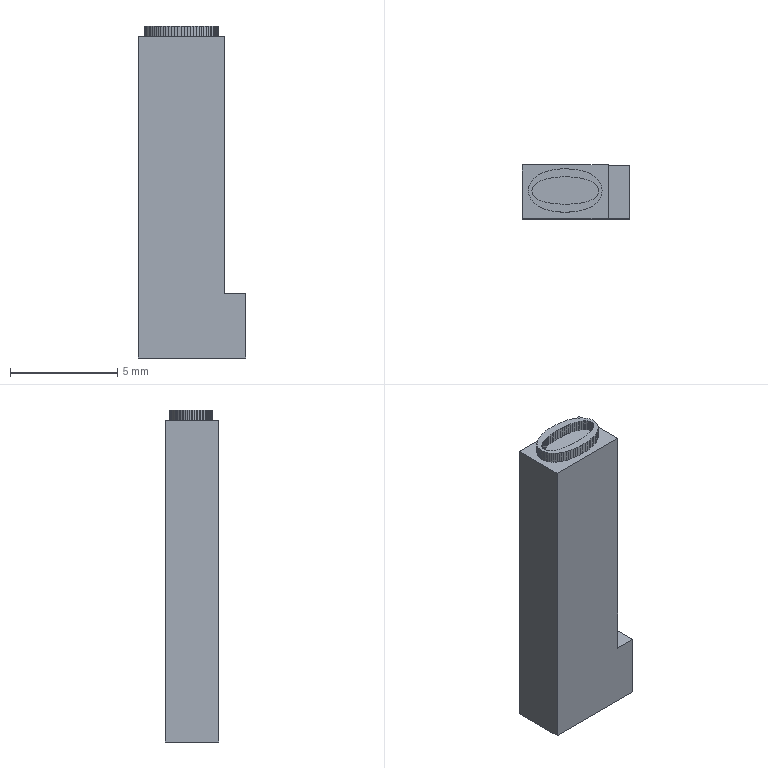Part | NX | features DIE-26 2 | 1 solid | 170 faces | box 5 x 2.5 x 15.5 mm | volume 158.679 mm3 | plane 170